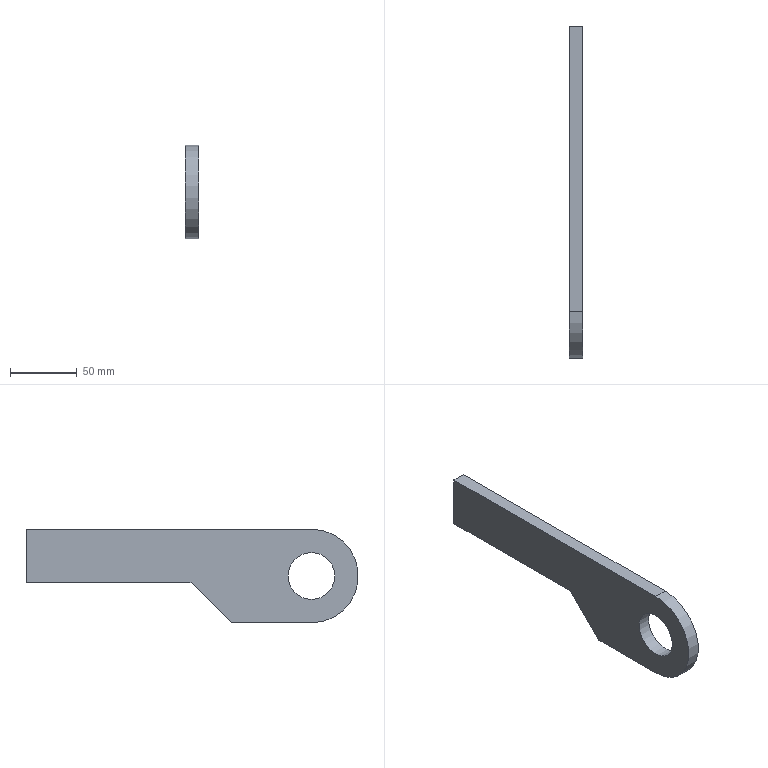Part | STEP file | body tilt cylinder mounting plate 2--000.001--20
240928 | 1 solid | 9 faces | box 10 x 248.257 x 70 mm | volume 117424 mm3 | plane 7 | cylinder 2 | commonest cylinder face diameters 35 x1 70 x1
STEP:
#1=CARTESIAN_POINT('',(0.,0.,0.));
#2=DIRECTION('',(0.,0.,1.));
#3=DIRECTION('',(1.,0.,0.));
#4=AXIS2_PLACEMENT_3D('',#1,#2,#3);
#5=CARTESIAN_POINT('',(-630.,216.,-35.));
#6=VERTEX_POINT('',#5);
#7=CARTESIAN_POINT('',(-630.,198.5,-35.));
#8=DIRECTION('',(1.,0.,0.));
#9=DIRECTION('',(0.,1.,0.));
#10=AXIS2_PLACEMENT_3D('',#7,#8,#9);
#11=CIRCLE('',#10,17.5);
#12=CARTESIAN_POINT('',(-630.,-284.,-150.));
#13=DIRECTION('',(1.,0.,0.));
#14=DIRECTION('',(0.,-1.,0.));
#15=AXIS2_PLACEMENT_3D('',#12,#13,#14);
#16=PLANE('',#15);
#17=CARTESIAN_POINT('',(-482.5,-115.));
#18=DIRECTION('',(-1.,0.));
#19=AXIS2_PLACEMENT_2D('',#17,#18);
#20=CIRCLE('',#19,17.5);
#21=(GEOMETRIC_REPRESENTATION_CONTEXT(2)PARAMETRIC_REPRESENTATION_CONTEXT()REPRESENTATION_CONTEXT('',''));
#22=DEFINITIONAL_REPRESENTATION('',(#20),#21);
#23=PCURVE('',#16,#22);
#24=CARTESIAN_POINT('',(-1050.,198.5,-35.));
#25=DIRECTION('',(1.,0.,0.));
#26=DIRECTION('',(0.,0.,1.));
#27=AXIS2_PLACEMENT_3D('',#24,#25,#26);
#28=CYLINDRICAL_SURFACE('',#27,17.5);
#29=CARTESIAN_POINT('',(4.712,420.));
#30=DIRECTION('',(1.,0.));
#31=VECTOR('',#30,1.);
#32=LINE('',#29,#31);
#33=(GEOMETRIC_REPRESENTATION_CONTEXT(2)PARAMETRIC_REPRESENTATION_CONTEXT()REPRESENTATION_CONTEXT('',''));
#34=DEFINITIONAL_REPRESENTATION('',(#32),#33);
#35=PCURVE('',#28,#34);
#36=SURFACE_CURVE('',#11,(#23,#35),.PCURVE_S1.);
#37=EDGE_CURVE('',#6,#6,#36,.T.);
#38=ORIENTED_EDGE('',*,*,#37,.F.);
#39=EDGE_LOOP('',(#38));
#40=FACE_BOUND('',#39,.T.);
#41=CARTESIAN_POINT('',(-630.,288.5,-40.));
#42=VERTEX_POINT('',#41);
#43=CARTESIAN_POINT('',(-630.,411.757,-40.));
#44=VERTEX_POINT('',#43);
#45=CARTESIAN_POINT('',(-630.,-284.,-40.));
#46=DIRECTION('',(0.,1.,0.));
#47=VECTOR('',#46,1.);
#48=LINE('',#45,#47);
#49=CARTESIAN_POINT('',(0.,-110.));
#50=DIRECTION('',(-1.,0.));
#51=VECTOR('',#50,1.);
#52=LINE('',#49,#51);
#53=(GEOMETRIC_REPRESENTATION_CONTEXT(2)PARAMETRIC_REPRESENTATION_CONTEXT()REPRESENTATION_CONTEXT('',''));
#54=DEFINITIONAL_REPRESENTATION('',(#52),#53);
#55=PCURVE('',#16,#54);
#56=CARTESIAN_POINT('',(-635.,288.5,-40.));
#57=DIRECTION('',(0.,0.,-1.));
#58=DIRECTION('',(1.,0.,0.));
#59=AXIS2_PLACEMENT_3D('',#56,#57,#58);
#60=PLANE('',#59);
#61=CARTESIAN_POINT('',(5.,572.5));
#62=DIRECTION('',(0.,-1.));
#63=VECTOR('',#62,1.);
#64=LINE('',#61,#63);
#65=(GEOMETRIC_REPRESENTATION_CONTEXT(2)PARAMETRIC_REPRESENTATION_CONTEXT()REPRESENTATION_CONTEXT('',''));
#66=DEFINITIONAL_REPRESENTATION('',(#64),#65);
#67=PCURVE('',#60,#66);
#68=SURFACE_CURVE('',#48,(#55,#67),.PCURVE_S1.);
#69=EDGE_CURVE('',#42,#44,#68,.T.);
#70=ORIENTED_EDGE('',*,*,#69,.T.);
#71=CARTESIAN_POINT('',(-630.,411.757,0.));
#72=VERTEX_POINT('',#71);
#73=CARTESIAN_POINT('',(-630.,411.757,-150.));
#74=DIRECTION('',(0.,0.,1.));
#75=VECTOR('',#74,1.);
#76=LINE('',#73,#75);
#77=CARTESIAN_POINT('',(-695.757,0.));
#78=DIRECTION('',(0.,-1.));
#79=VECTOR('',#78,1.);
#80=LINE('',#77,#79);
#81=(GEOMETRIC_REPRESENTATION_CONTEXT(2)PARAMETRIC_REPRESENTATION_CONTEXT()REPRESENTATION_CONTEXT('',''));
#82=DEFINITIONAL_REPRESENTATION('',(#80),#81);
#83=PCURVE('',#16,#82);
#84=CARTESIAN_POINT('',(-640.,411.757,0.));
#85=DIRECTION('',(0.,1.,0.));
#86=DIRECTION('',(0.,0.,-1.));
#87=AXIS2_PLACEMENT_3D('',#84,#85,#86);
#88=PLANE('',#87);
#89=CARTESIAN_POINT('',(150.,-10.));
#90=DIRECTION('',(-1.,0.));
#91=VECTOR('',#90,1.);
#92=LINE('',#89,#91);
#93=(GEOMETRIC_REPRESENTATION_CONTEXT(2)PARAMETRIC_REPRESENTATION_CONTEXT()REPRESENTATION_CONTEXT('',''));
#94=DEFINITIONAL_REPRESENTATION('',(#92),#93);
#95=PCURVE('',#88,#94);
#96=SURFACE_CURVE('',#76,(#83,#95),.PCURVE_S1.);
#97=EDGE_CURVE('',#44,#72,#96,.T.);
#98=ORIENTED_EDGE('',*,*,#97,.T.);
#99=CARTESIAN_POINT('',(-630.,198.5,0.));
#100=VERTEX_POINT('',#99);
#101=CARTESIAN_POINT('',(-630.,-488.,0.));
#102=DIRECTION('',(0.,1.,0.));
#103=VECTOR('',#102,1.);
#104=LINE('',#101,#103);
#105=CARTESIAN_POINT('',(204.,-150.));
#106=DIRECTION('',(-1.,0.));
#107=VECTOR('',#106,1.);
#108=LINE('',#105,#107);
#109=(GEOMETRIC_REPRESENTATION_CONTEXT(2)PARAMETRIC_REPRESENTATION_CONTEXT()REPRESENTATION_CONTEXT('',''));
#110=DEFINITIONAL_REPRESENTATION('',(#108),#109);
#111=PCURVE('',#16,#110);
#112=CARTESIAN_POINT('',(-750.,-488.,0.));
#113=DIRECTION('',(0.,0.,1.));
#114=DIRECTION('',(0.,1.,0.));
#115=AXIS2_PLACEMENT_3D('',#112,#113,#114);
#116=PLANE('',#115);
#117=CARTESIAN_POINT('',(0.,-120.));
#118=DIRECTION('',(1.,0.));
#119=VECTOR('',#118,1.);
#120=LINE('',#117,#119);
#121=(GEOMETRIC_REPRESENTATION_CONTEXT(2)PARAMETRIC_REPRESENTATION_CONTEXT()REPRESENTATION_CONTEXT('',''));
#122=DEFINITIONAL_REPRESENTATION('',(#120),#121);
#123=PCURVE('',#116,#122);
#124=SURFACE_CURVE('',#104,(#111,#123),.PCURVE_S1.);
#125=EDGE_CURVE('',#100,#72,#124,.T.);
#126=ORIENTED_EDGE('',*,*,#125,.F.);
#127=CARTESIAN_POINT('',(-630.,198.5,-70.));
#128=VERTEX_POINT('',#127);
#129=CARTESIAN_POINT('',(-630.,198.5,-35.));
#130=DIRECTION('',(1.,0.,0.));
#131=DIRECTION('',(0.,1.,0.));
#132=AXIS2_PLACEMENT_3D('',#129,#130,#131);
#133=CIRCLE('',#132,35.);
#134=CARTESIAN_POINT('',(-482.5,-115.));
#135=DIRECTION('',(-1.,0.));
#136=AXIS2_PLACEMENT_2D('',#134,#135);
#137=CIRCLE('',#136,35.);
#138=(GEOMETRIC_REPRESENTATION_CONTEXT(2)PARAMETRIC_REPRESENTATION_CONTEXT()REPRESENTATION_CONTEXT('',''));
#139=DEFINITIONAL_REPRESENTATION('',(#137),#138);
#140=PCURVE('',#16,#139);
#141=CARTESIAN_POINT('',(-700.,198.5,-35.));
#142=DIRECTION('',(-1.,0.,0.));
#143=DIRECTION('',(0.,0.,-1.));
#144=AXIS2_PLACEMENT_3D('',#141,#142,#143);
#145=CYLINDRICAL_SURFACE('',#144,35.);
#146=CARTESIAN_POINT('',(4.712,-70.));
#147=DIRECTION('',(-1.,0.));
#148=VECTOR('',#147,1.);
#149=LINE('',#146,#148);
#150=(GEOMETRIC_REPRESENTATION_CONTEXT(2)PARAMETRIC_REPRESENTATION_CONTEXT()REPRESENTATION_CONTEXT('',''));
#151=DEFINITIONAL_REPRESENTATION('',(#149),#150);
#152=PCURVE('',#145,#151);
#153=SURFACE_CURVE('',#133,(#140,#152),.PCURVE_S1.);
#154=EDGE_CURVE('',#100,#128,#153,.T.);
#155=ORIENTED_EDGE('',*,*,#154,.T.);
#156=CARTESIAN_POINT('',(-630.,258.5,-70.));
#157=VERTEX_POINT('',#156);
#158=CARTESIAN_POINT('',(-630.,198.5,-70.));
#159=DIRECTION('',(0.,-1.,0.));
#160=VECTOR('',#159,1.);
#161=LINE('',#158,#160);
#162=CARTESIAN_POINT('',(-482.5,-80.));
#163=DIRECTION('',(1.,0.));
#164=VECTOR('',#163,1.);
#165=LINE('',#162,#164);
#166=(GEOMETRIC_REPRESENTATION_CONTEXT(2)PARAMETRIC_REPRESENTATION_CONTEXT()REPRESENTATION_CONTEXT('',''));
#167=DEFINITIONAL_REPRESENTATION('',(#165),#166);
#168=PCURVE('',#16,#167);
#169=CARTESIAN_POINT('',(-700.,198.5,-70.));
#170=DIRECTION('',(0.,0.,-1.));
#171=DIRECTION('',(1.,0.,0.));
#172=AXIS2_PLACEMENT_3D('',#169,#170,#171);
#173=PLANE('',#172);
#174=CARTESIAN_POINT('',(70.,0.));
#175=DIRECTION('',(0.,1.));
#176=VECTOR('',#175,1.);
#177=LINE('',#174,#176);
#178=(GEOMETRIC_REPRESENTATION_CONTEXT(2)PARAMETRIC_REPRESENTATION_CONTEXT()REPRESENTATION_CONTEXT('',''));
#179=DEFINITIONAL_REPRESENTATION('',(#177),#178);
#180=PCURVE('',#173,#179);
#181=SURFACE_CURVE('',#161,(#168,#180),.PCURVE_S1.);
#182=EDGE_CURVE('',#157,#128,#181,.T.);
#183=ORIENTED_EDGE('',*,*,#182,.F.);
#184=CARTESIAN_POINT('',(-630.,-102.75,-431.25));
#185=DIRECTION('',(0.,0.7071,0.7071));
#186=VECTOR('',#185,1.);
#187=LINE('',#184,#186);
#188=CARTESIAN_POINT('',(-181.25,281.25));
#189=DIRECTION('',(-0.7071,-0.7071));
#190=VECTOR('',#189,1.);
#191=LINE('',#188,#190);
#192=(GEOMETRIC_REPRESENTATION_CONTEXT(2)PARAMETRIC_REPRESENTATION_CONTEXT()REPRESENTATION_CONTEXT('',''));
#193=DEFINITIONAL_REPRESENTATION('',(#191),#192);
#194=PCURVE('',#16,#193);
#195=CARTESIAN_POINT('',(600.173,268.5,-60.));
#196=DIRECTION('',(0.,-0.7071,0.7071));
#197=DIRECTION('',(1.,0.,0.));
#198=AXIS2_PLACEMENT_3D('',#195,#196,#197);
#199=PLANE('',#198);
#200=CARTESIAN_POINT('',(-1230.173,-525.027));
#201=DIRECTION('',(0.,1.));
#202=VECTOR('',#201,1.);
#203=LINE('',#200,#202);
#204=(GEOMETRIC_REPRESENTATION_CONTEXT(2)PARAMETRIC_REPRESENTATION_CONTEXT()REPRESENTATION_CONTEXT('',''));
#205=DEFINITIONAL_REPRESENTATION('',(#203),#204);
#206=PCURVE('',#199,#205);
#207=SURFACE_CURVE('',#187,(#194,#206),.PCURVE_S1.);
#208=EDGE_CURVE('',#157,#42,#207,.T.);
#209=ORIENTED_EDGE('',*,*,#208,.T.);
#210=EDGE_LOOP('',(#70,#98,#126,#155,#183,#209));
#211=FACE_BOUND('',#210,.T.);
#212=ADVANCED_FACE('',(#40,#211),#16,.T.);
#213=ORIENTED_EDGE('',*,*,#125,.T.);
#214=CARTESIAN_POINT('',(-640.,411.757,0.));
#215=VERTEX_POINT('',#214);
#216=CARTESIAN_POINT('',(-750.,411.757,0.));
#217=DIRECTION('',(-1.,0.,0.));
#218=VECTOR('',#217,1.);
#219=LINE('',#216,#218);
#220=CARTESIAN_POINT('',(899.757,0.));
#221=DIRECTION('',(0.,1.));
#222=VECTOR('',#221,1.);
#223=LINE('',#220,#222);
#224=(GEOMETRIC_REPRESENTATION_CONTEXT(2)PARAMETRIC_REPRESENTATION_CONTEXT()REPRESENTATION_CONTEXT('',''));
#225=DEFINITIONAL_REPRESENTATION('',(#223),#224);
#226=PCURVE('',#116,#225);
#227=CARTESIAN_POINT('',(0.,110.));
#228=DIRECTION('',(0.,1.));
#229=VECTOR('',#228,1.);
#230=LINE('',#227,#229);
#231=(GEOMETRIC_REPRESENTATION_CONTEXT(2)PARAMETRIC_REPRESENTATION_CONTEXT()REPRESENTATION_CONTEXT('',''));
#232=DEFINITIONAL_REPRESENTATION('',(#230),#231);
#233=PCURVE('',#88,#232);
#234=SURFACE_CURVE('',#219,(#226,#233),.PCURVE_S1.);
#235=EDGE_CURVE('',#72,#215,#234,.T.);
#236=ORIENTED_EDGE('',*,*,#235,.T.);
#237=CARTESIAN_POINT('',(-640.,198.5,0.));
#238=VERTEX_POINT('',#237);
#239=CARTESIAN_POINT('',(-640.,-488.,0.));
#240=DIRECTION('',(0.,-1.,0.));
#241=VECTOR('',#240,1.);
#242=LINE('',#239,#241);
#243=CARTESIAN_POINT('',(0.,-110.));
#244=DIRECTION('',(-1.,0.));
#245=VECTOR('',#244,1.);
#246=LINE('',#243,#245);
#247=(GEOMETRIC_REPRESENTATION_CONTEXT(2)PARAMETRIC_REPRESENTATION_CONTEXT()REPRESENTATION_CONTEXT('',''));
#248=DEFINITIONAL_REPRESENTATION('',(#246),#247);
#249=PCURVE('',#116,#248);
#250=CARTESIAN_POINT('',(-640.,-284.,-150.));
#251=DIRECTION('',(-1.,0.,0.));
#252=DIRECTION('',(0.,1.,0.));
#253=AXIS2_PLACEMENT_3D('',#250,#251,#252);
#254=PLANE('',#253);
#255=CARTESIAN_POINT('',(-204.,-150.));
#256=DIRECTION('',(-1.,0.));
#257=VECTOR('',#256,1.);
#258=LINE('',#255,#257);
#259=(GEOMETRIC_REPRESENTATION_CONTEXT(2)PARAMETRIC_REPRESENTATION_CONTEXT()REPRESENTATION_CONTEXT('',''));
#260=DEFINITIONAL_REPRESENTATION('',(#258),#259);
#261=PCURVE('',#254,#260);
#262=SURFACE_CURVE('',#242,(#249,#261),.PCURVE_S1.);
#263=EDGE_CURVE('',#215,#238,#262,.T.);
#264=ORIENTED_EDGE('',*,*,#263,.T.);
#265=CARTESIAN_POINT('',(-750.,198.5,0.));
#266=DIRECTION('',(1.,0.,0.));
#267=VECTOR('',#266,1.);
#268=LINE('',#265,#267);
#269=CARTESIAN_POINT('',(686.5,0.));
#270=DIRECTION('',(0.,-1.));
#271=VECTOR('',#270,1.);
#272=LINE('',#269,#271);
#273=(GEOMETRIC_REPRESENTATION_CONTEXT(2)PARAMETRIC_REPRESENTATION_CONTEXT()REPRESENTATION_CONTEXT('',''));
#274=DEFINITIONAL_REPRESENTATION('',(#272),#273);
#275=PCURVE('',#116,#274);
#276=CARTESIAN_POINT('',(3.142,50.));
#277=DIRECTION('',(0.,-1.));
#278=VECTOR('',#277,1.);
#279=LINE('',#276,#278);
#280=(GEOMETRIC_REPRESENTATION_CONTEXT(2)PARAMETRIC_REPRESENTATION_CONTEXT()REPRESENTATION_CONTEXT('',''));
#281=DEFINITIONAL_REPRESENTATION('',(#279),#280);
#282=PCURVE('',#145,#281);
#283=SURFACE_CURVE('',#268,(#275,#282),.PCURVE_S1.);
#284=EDGE_CURVE('',#238,#100,#283,.T.);
#285=ORIENTED_EDGE('',*,*,#284,.T.);
#286=EDGE_LOOP('',(#213,#236,#264,#285));
#287=FACE_BOUND('',#286,.T.);
#288=ADVANCED_FACE('',(#287),#116,.T.);
#289=CARTESIAN_POINT('',(-640.,411.757,-40.));
#290=VERTEX_POINT('',#289);
#291=CARTESIAN_POINT('',(-640.,288.5,-40.));
#292=VERTEX_POINT('',#291);
#293=CARTESIAN_POINT('',(-640.,-284.,-40.));
#294=DIRECTION('',(0.,-1.,0.));
#295=VECTOR('',#294,1.);
#296=LINE('',#293,#295);
#297=CARTESIAN_POINT('',(-5.,572.5));
#298=DIRECTION('',(0.,1.));
#299=VECTOR('',#298,1.);
#300=LINE('',#297,#299);
#301=(GEOMETRIC_REPRESENTATION_CONTEXT(2)PARAMETRIC_REPRESENTATION_CONTEXT()REPRESENTATION_CONTEXT('',''));
#302=DEFINITIONAL_REPRESENTATION('',(#300),#301);
#303=PCURVE('',#60,#302);
#304=CARTESIAN_POINT('',(0.,-110.));
#305=DIRECTION('',(-1.,0.));
#306=VECTOR('',#305,1.);
#307=LINE('',#304,#306);
#308=(GEOMETRIC_REPRESENTATION_CONTEXT(2)PARAMETRIC_REPRESENTATION_CONTEXT()REPRESENTATION_CONTEXT('',''));
#309=DEFINITIONAL_REPRESENTATION('',(#307),#308);
#310=PCURVE('',#254,#309);
#311=SURFACE_CURVE('',#296,(#303,#310),.PCURVE_S1.);
#312=EDGE_CURVE('',#290,#292,#311,.T.);
#313=ORIENTED_EDGE('',*,*,#312,.F.);
#314=CARTESIAN_POINT('',(-635.,411.757,-40.));
#315=DIRECTION('',(1.,0.,0.));
#316=VECTOR('',#315,1.);
#317=LINE('',#314,#316);
#318=CARTESIAN_POINT('',(0.,-123.257));
#319=DIRECTION('',(1.,0.));
#320=VECTOR('',#319,1.);
#321=LINE('',#318,#320);
#322=(GEOMETRIC_REPRESENTATION_CONTEXT(2)PARAMETRIC_REPRESENTATION_CONTEXT()REPRESENTATION_CONTEXT('',''));
#323=DEFINITIONAL_REPRESENTATION('',(#321),#322);
#324=PCURVE('',#60,#323);
#325=CARTESIAN_POINT('',(40.,-5.));
#326=DIRECTION('',(0.,-1.));
#327=VECTOR('',#326,1.);
#328=LINE('',#325,#327);
#329=(GEOMETRIC_REPRESENTATION_CONTEXT(2)PARAMETRIC_REPRESENTATION_CONTEXT()REPRESENTATION_CONTEXT('',''));
#330=DEFINITIONAL_REPRESENTATION('',(#328),#329);
#331=PCURVE('',#88,#330);
#332=SURFACE_CURVE('',#317,(#324,#331),.PCURVE_S1.);
#333=EDGE_CURVE('',#290,#44,#332,.T.);
#334=ORIENTED_EDGE('',*,*,#333,.T.);
#335=ORIENTED_EDGE('',*,*,#69,.F.);
#336=CARTESIAN_POINT('',(-635.,288.5,-40.));
#337=DIRECTION('',(1.,0.,0.));
#338=VECTOR('',#337,1.);
#339=LINE('',#336,#338);
#340=CARTESIAN_POINT('',(0.,0.));
#341=DIRECTION('',(1.,0.));
#342=VECTOR('',#341,1.);
#343=LINE('',#340,#342);
#344=(GEOMETRIC_REPRESENTATION_CONTEXT(2)PARAMETRIC_REPRESENTATION_CONTEXT()REPRESENTATION_CONTEXT('',''));
#345=DEFINITIONAL_REPRESENTATION('',(#343),#344);
#346=PCURVE('',#60,#345);
#347=CARTESIAN_POINT('',(-1235.173,28.284));
#348=DIRECTION('',(1.,0.));
#349=VECTOR('',#348,1.);
#350=LINE('',#347,#349);
#351=(GEOMETRIC_REPRESENTATION_CONTEXT(2)PARAMETRIC_REPRESENTATION_CONTEXT()REPRESENTATION_CONTEXT('',''));
#352=DEFINITIONAL_REPRESENTATION('',(#350),#351);
#353=PCURVE('',#199,#352);
#354=SURFACE_CURVE('',#339,(#346,#353),.PCURVE_S1.);
#355=EDGE_CURVE('',#292,#42,#354,.T.);
#356=ORIENTED_EDGE('',*,*,#355,.F.);
#357=EDGE_LOOP('',(#313,#334,#335,#356));
#358=FACE_BOUND('',#357,.T.);
#359=ADVANCED_FACE('',(#358),#60,.T.);
#360=CARTESIAN_POINT('',(-640.,181.,-35.));
#361=VERTEX_POINT('',#360);
#362=CARTESIAN_POINT('',(-640.,216.,-35.));
#363=VERTEX_POINT('',#362);
#364=CARTESIAN_POINT('',(-640.,198.5,-35.));
#365=DIRECTION('',(-1.,0.,0.));
#366=DIRECTION('',(0.,-1.,0.));
#367=AXIS2_PLACEMENT_3D('',#364,#365,#366);
#368=CIRCLE('',#367,17.5);
#369=CARTESIAN_POINT('',(482.5,-115.));
#370=DIRECTION('',(-1.,0.));
#371=AXIS2_PLACEMENT_2D('',#369,#370);
#372=CIRCLE('',#371,17.5);
#373=(GEOMETRIC_REPRESENTATION_CONTEXT(2)PARAMETRIC_REPRESENTATION_CONTEXT()REPRESENTATION_CONTEXT('',''));
#374=DEFINITIONAL_REPRESENTATION('',(#372),#373);
#375=PCURVE('',#254,#374);
#376=CARTESIAN_POINT('',(7.854,410.));
#377=DIRECTION('',(-1.,0.));
#378=VECTOR('',#377,1.);
#379=LINE('',#376,#378);
#380=(GEOMETRIC_REPRESENTATION_CONTEXT(2)PARAMETRIC_REPRESENTATION_CONTEXT()REPRESENTATION_CONTEXT('',''));
#381=DEFINITIONAL_REPRESENTATION('',(#379),#380);
#382=PCURVE('',#28,#381);
#383=SURFACE_CURVE('',#368,(#375,#382),.PCURVE_S1.);
#384=EDGE_CURVE('',#361,#363,#383,.T.);
#385=ORIENTED_EDGE('',*,*,#384,.F.);
#386=CARTESIAN_POINT('',(-640.,198.5,-35.));
#387=DIRECTION('',(-1.,0.,0.));
#388=DIRECTION('',(0.,-1.,0.));
#389=AXIS2_PLACEMENT_3D('',#386,#387,#388);
#390=CIRCLE('',#389,17.5);
#391=CARTESIAN_POINT('',(482.5,-115.));
#392=DIRECTION('',(-1.,0.));
#393=AXIS2_PLACEMENT_2D('',#391,#392);
#394=CIRCLE('',#393,17.5);
#395=(GEOMETRIC_REPRESENTATION_CONTEXT(2)PARAMETRIC_REPRESENTATION_CONTEXT()REPRESENTATION_CONTEXT('',''));
#396=DEFINITIONAL_REPRESENTATION('',(#394),#395);
#397=PCURVE('',#254,#396);
#398=CARTESIAN_POINT('',(14.137,410.));
#399=DIRECTION('',(-1.,0.));
#400=VECTOR('',#399,1.);
#401=LINE('',#398,#400);
#402=(GEOMETRIC_REPRESENTATION_CONTEXT(2)PARAMETRIC_REPRESENTATION_CONTEXT()REPRESENTATION_CONTEXT('',''));
#403=DEFINITIONAL_REPRESENTATION('',(#401),#402);
#404=PCURVE('',#28,#403);
#405=SURFACE_CURVE('',#390,(#397,#404),.PCURVE_S1.);
#406=EDGE_CURVE('',#363,#361,#405,.T.);
#407=ORIENTED_EDGE('',*,*,#406,.F.);
#408=EDGE_LOOP('',(#385,#407));
#409=FACE_BOUND('',#408,.T.);
#410=CARTESIAN_POINT('',(-640.,411.757,0.000000001));
#411=DIRECTION('',(0.,0.,1.));
#412=VECTOR('',#411,1.);
#413=LINE('',#410,#412);
#414=CARTESIAN_POINT('',(695.757,-150.));
#415=DIRECTION('',(0.,-1.));
#416=VECTOR('',#415,1.);
#417=LINE('',#414,#416);
#418=(GEOMETRIC_REPRESENTATION_CONTEXT(2)PARAMETRIC_REPRESENTATION_CONTEXT()REPRESENTATION_CONTEXT('',''));
#419=DEFINITIONAL_REPRESENTATION('',(#417),#418);
#420=PCURVE('',#254,#419);
#421=CARTESIAN_POINT('',(-0.000000001,0.));
#422=DIRECTION('',(-1.,0.));
#423=VECTOR('',#422,1.);
#424=LINE('',#421,#423);
#425=(GEOMETRIC_REPRESENTATION_CONTEXT(2)PARAMETRIC_REPRESENTATION_CONTEXT()REPRESENTATION_CONTEXT('',''));
#426=DEFINITIONAL_REPRESENTATION('',(#424),#425);
#427=PCURVE('',#88,#426);
#428=SURFACE_CURVE('',#413,(#420,#427),.PCURVE_S1.);
#429=EDGE_CURVE('',#290,#215,#428,.T.);
#430=ORIENTED_EDGE('',*,*,#429,.F.);
#431=ORIENTED_EDGE('',*,*,#312,.T.);
#432=CARTESIAN_POINT('',(-640.,258.5,-70.));
#433=VERTEX_POINT('',#432);
#434=CARTESIAN_POINT('',(-640.,-102.75,-431.25));
#435=DIRECTION('',(0.,-0.7071,-0.7071));
#436=VECTOR('',#435,1.);
#437=LINE('',#434,#436);
#438=CARTESIAN_POINT('',(181.25,281.25));
#439=DIRECTION('',(-0.7071,0.7071));
#440=VECTOR('',#439,1.);
#441=LINE('',#438,#440);
#442=(GEOMETRIC_REPRESENTATION_CONTEXT(2)PARAMETRIC_REPRESENTATION_CONTEXT()REPRESENTATION_CONTEXT('',''));
#443=DEFINITIONAL_REPRESENTATION('',(#441),#442);
#444=PCURVE('',#254,#443);
#445=CARTESIAN_POINT('',(-1240.173,-525.027));
#446=DIRECTION('',(0.,-1.));
#447=VECTOR('',#446,1.);
#448=LINE('',#445,#447);
#449=(GEOMETRIC_REPRESENTATION_CONTEXT(2)PARAMETRIC_REPRESENTATION_CONTEXT()REPRESENTATION_CONTEXT('',''));
#450=DEFINITIONAL_REPRESENTATION('',(#448),#449);
#451=PCURVE('',#199,#450);
#452=SURFACE_CURVE('',#437,(#444,#451),.PCURVE_S1.);
#453=EDGE_CURVE('',#292,#433,#452,.T.);
#454=ORIENTED_EDGE('',*,*,#453,.T.);
#455=CARTESIAN_POINT('',(-640.,198.5,-70.));
#456=VERTEX_POINT('',#455);
#457=CARTESIAN_POINT('',(-640.,198.5,-70.));
#458=DIRECTION('',(0.,1.,0.));
#459=VECTOR('',#458,1.);
#460=LINE('',#457,#459);
#461=CARTESIAN_POINT('',(482.5,-80.));
#462=DIRECTION('',(1.,0.));
#463=VECTOR('',#462,1.);
#464=LINE('',#461,#463);
#465=(GEOMETRIC_REPRESENTATION_CONTEXT(2)PARAMETRIC_REPRESENTATION_CONTEXT()REPRESENTATION_CONTEXT('',''));
#466=DEFINITIONAL_REPRESENTATION('',(#464),#465);
#467=PCURVE('',#254,#466);
#468=CARTESIAN_POINT('',(60.,0.));
#469=DIRECTION('',(0.,-1.));
#470=VECTOR('',#469,1.);
#471=LINE('',#468,#470);
#472=(GEOMETRIC_REPRESENTATION_CONTEXT(2)PARAMETRIC_REPRESENTATION_CONTEXT()REPRESENTATION_CONTEXT('',''));
#473=DEFINITIONAL_REPRESENTATION('',(#471),#472);
#474=PCURVE('',#173,#473);
#475=SURFACE_CURVE('',#460,(#467,#474),.PCURVE_S1.);
#476=EDGE_CURVE('',#456,#433,#475,.T.);
#477=ORIENTED_EDGE('',*,*,#476,.F.);
#478=CARTESIAN_POINT('',(-640.,198.5,-35.));
#479=DIRECTION('',(-1.,0.,0.));
#480=DIRECTION('',(0.,-1.,0.));
#481=AXIS2_PLACEMENT_3D('',#478,#479,#480);
#482=CIRCLE('',#481,35.);
#483=CARTESIAN_POINT('',(482.5,-115.));
#484=DIRECTION('',(-1.,0.));
#485=AXIS2_PLACEMENT_2D('',#483,#484);
#486=CIRCLE('',#485,35.);
#487=(GEOMETRIC_REPRESENTATION_CONTEXT(2)PARAMETRIC_REPRESENTATION_CONTEXT()REPRESENTATION_CONTEXT('',''));
#488=DEFINITIONAL_REPRESENTATION('',(#486),#487);
#489=PCURVE('',#254,#488);
#490=CARTESIAN_POINT('',(-4.712,-60.));
#491=DIRECTION('',(1.,0.));
#492=VECTOR('',#491,1.);
#493=LINE('',#490,#492);
#494=(GEOMETRIC_REPRESENTATION_CONTEXT(2)PARAMETRIC_REPRESENTATION_CONTEXT()REPRESENTATION_CONTEXT('',''));
#495=DEFINITIONAL_REPRESENTATION('',(#493),#494);
#496=PCURVE('',#145,#495);
#497=SURFACE_CURVE('',#482,(#489,#496),.PCURVE_S1.);
#498=EDGE_CURVE('',#456,#238,#497,.T.);
#499=ORIENTED_EDGE('',*,*,#498,.T.);
#500=ORIENTED_EDGE('',*,*,#263,.F.);
#501=EDGE_LOOP('',(#430,#431,#454,#477,#499,#500));
#502=FACE_BOUND('',#501,.T.);
#503=ADVANCED_FACE('',(#409,#502),#254,.T.);
#504=ORIENTED_EDGE('',*,*,#498,.F.);
#505=CARTESIAN_POINT('',(-700.,198.5,-70.));
#506=DIRECTION('',(-1.,0.,0.));
#507=VECTOR('',#506,1.);
#508=LINE('',#505,#507);
#509=CARTESIAN_POINT('',(0.,0.));
#510=DIRECTION('',(0.,1.));
#511=VECTOR('',#510,1.);
#512=LINE('',#509,#511);
#513=(GEOMETRIC_REPRESENTATION_CONTEXT(2)PARAMETRIC_REPRESENTATION_CONTEXT()REPRESENTATION_CONTEXT('',''));
#514=DEFINITIONAL_REPRESENTATION('',(#512),#513);
#515=PCURVE('',#145,#514);
#516=CARTESIAN_POINT('',(0.,0.));
#517=DIRECTION('',(-1.,0.));
#518=VECTOR('',#517,1.);
#519=LINE('',#516,#518);
#520=(GEOMETRIC_REPRESENTATION_CONTEXT(2)PARAMETRIC_REPRESENTATION_CONTEXT()REPRESENTATION_CONTEXT('',''));
#521=DEFINITIONAL_REPRESENTATION('',(#519),#520);
#522=PCURVE('',#173,#521);
#523=SURFACE_CURVE('',#508,(#515,#522),.PCURVE_S1.);
#524=EDGE_CURVE('',#128,#456,#523,.T.);
#525=ORIENTED_EDGE('',*,*,#524,.F.);
#526=ORIENTED_EDGE('',*,*,#154,.F.);
#527=ORIENTED_EDGE('',*,*,#284,.F.);
#528=EDGE_LOOP('',(#504,#525,#526,#527));
#529=FACE_BOUND('',#528,.T.);
#530=ADVANCED_FACE('',(#529),#145,.T.);
#531=ORIENTED_EDGE('',*,*,#406,.F.);
#532=CARTESIAN_POINT('',(-640.,216.,-35.));
#533=CARTESIAN_POINT('',(-630.,216.,-35.));
#534=B_SPLINE_CURVE_WITH_KNOTS('',1,(#532,#533),.UNSPECIFIED.,.F.,.F.,(2,2),(410.,420.),.PIECEWISE_BEZIER_KNOTS.);
#535=CARTESIAN_POINT('',(10.996,0.));
#536=DIRECTION('',(0.,1.));
#537=VECTOR('',#536,1.);
#538=LINE('',#535,#537);
#539=(GEOMETRIC_REPRESENTATION_CONTEXT(2)PARAMETRIC_REPRESENTATION_CONTEXT()REPRESENTATION_CONTEXT('',''));
#540=DEFINITIONAL_REPRESENTATION('',(#538),#539);
#541=PCURVE('',#28,#540);
#542=CARTESIAN_POINT('',(4.712,0.));
#543=DIRECTION('',(0.,1.));
#544=VECTOR('',#543,1.);
#545=LINE('',#542,#544);
#546=(GEOMETRIC_REPRESENTATION_CONTEXT(2)PARAMETRIC_REPRESENTATION_CONTEXT()REPRESENTATION_CONTEXT('',''));
#547=DEFINITIONAL_REPRESENTATION('',(#545),#546);
#548=PCURVE('',#28,#547);
#549=SEAM_CURVE('',#534,(#541,#548),.PCURVE_S1.);
#550=EDGE_CURVE('',#363,#6,#549,.T.);
#551=ORIENTED_EDGE('',*,*,#550,.T.);
#552=ORIENTED_EDGE('',*,*,#37,.F.);
#553=ORIENTED_EDGE('',*,*,#550,.F.);
#554=ORIENTED_EDGE('',*,*,#384,.F.);
#555=EDGE_LOOP('',(#531,#551,#552,#553,#554));
#556=FACE_BOUND('',#555,.F.);
#557=ADVANCED_FACE('',(#556),#28,.F.);
#558=ORIENTED_EDGE('',*,*,#476,.T.);
#559=CARTESIAN_POINT('',(-700.,258.5,-70.));
#560=DIRECTION('',(1.,0.,0.));
#561=VECTOR('',#560,1.);
#562=LINE('',#559,#561);
#563=CARTESIAN_POINT('',(0.,-60.));
#564=DIRECTION('',(1.,0.));
#565=VECTOR('',#564,1.);
#566=LINE('',#563,#565);
#567=(GEOMETRIC_REPRESENTATION_CONTEXT(2)PARAMETRIC_REPRESENTATION_CONTEXT()REPRESENTATION_CONTEXT('',''));
#568=DEFINITIONAL_REPRESENTATION('',(#566),#567);
#569=PCURVE('',#173,#568);
#570=CARTESIAN_POINT('',(-1300.173,-14.142));
#571=DIRECTION('',(1.,0.));
#572=VECTOR('',#571,1.);
#573=LINE('',#570,#572);
#574=(GEOMETRIC_REPRESENTATION_CONTEXT(2)PARAMETRIC_REPRESENTATION_CONTEXT()REPRESENTATION_CONTEXT('',''));
#575=DEFINITIONAL_REPRESENTATION('',(#573),#574);
#576=PCURVE('',#199,#575);
#577=SURFACE_CURVE('',#562,(#569,#576),.PCURVE_S1.);
#578=EDGE_CURVE('',#433,#157,#577,.T.);
#579=ORIENTED_EDGE('',*,*,#578,.T.);
#580=ORIENTED_EDGE('',*,*,#182,.T.);
#581=ORIENTED_EDGE('',*,*,#524,.T.);
#582=EDGE_LOOP('',(#558,#579,#580,#581));
#583=FACE_BOUND('',#582,.T.);
#584=ADVANCED_FACE('',(#583),#173,.T.);
#585=ORIENTED_EDGE('',*,*,#208,.F.);
#586=ORIENTED_EDGE('',*,*,#578,.F.);
#587=ORIENTED_EDGE('',*,*,#453,.F.);
#588=ORIENTED_EDGE('',*,*,#355,.T.);
#589=EDGE_LOOP('',(#585,#586,#587,#588));
#590=FACE_BOUND('',#589,.T.);
#591=ADVANCED_FACE('',(#590),#199,.F.);
#592=ORIENTED_EDGE('',*,*,#97,.F.);
#593=ORIENTED_EDGE('',*,*,#333,.F.);
#594=ORIENTED_EDGE('',*,*,#429,.T.);
#595=ORIENTED_EDGE('',*,*,#235,.F.);
#596=EDGE_LOOP('',(#592,#593,#594,#595));
#597=FACE_BOUND('',#596,.T.);
#598=ADVANCED_FACE('',(#597),#88,.T.);
#599=CLOSED_SHELL('',(#212,#288,#359,#503,#530,#557,#584,#591,#598));
#600=MANIFOLD_SOLID_BREP('',#599);
#601=(LENGTH_UNIT()NAMED_UNIT(*)SI_UNIT(.MILLI.,.METRE.));
#602=UNCERTAINTY_MEASURE_WITH_UNIT(LENGTH_MEASURE(0.000001),#601,'','');
#603=(NAMED_UNIT(*)PLANE_ANGLE_UNIT()SI_UNIT($,.RADIAN.));
#604=(NAMED_UNIT(*)SI_UNIT($,.STERADIAN.)SOLID_ANGLE_UNIT());
#605=(GEOMETRIC_REPRESENTATION_CONTEXT(3)GLOBAL_UNCERTAINTY_ASSIGNED_CONTEXT((#602))GLOBAL_UNIT_ASSIGNED_CONTEXT((#601,#603,#604))REPRESENTATION_CONTEXT('',''));
#606=ADVANCED_BREP_SHAPE_REPRESENTATION('',(#4,#600),#605);